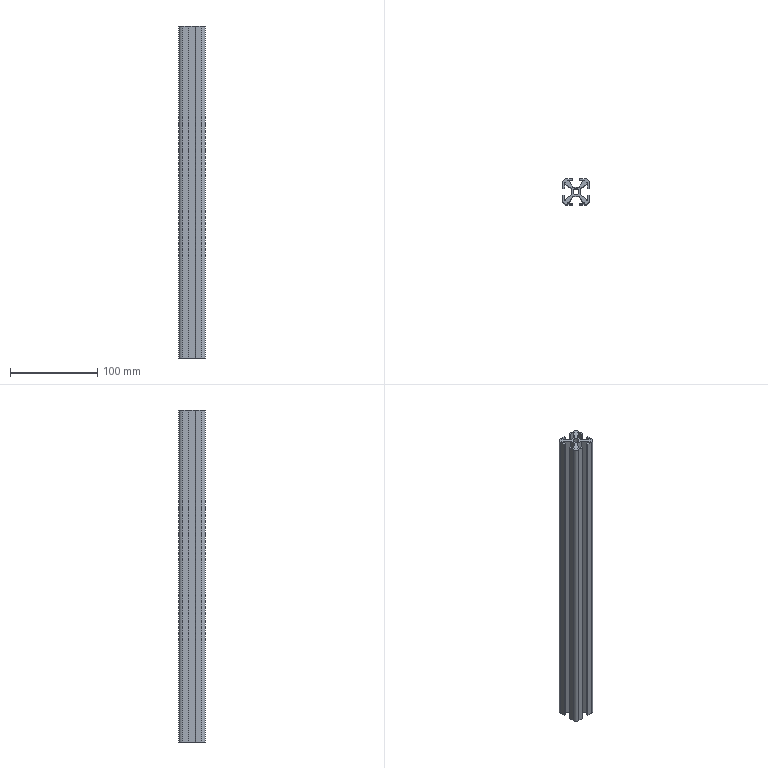Part | SolidWorks | features CirPattern 1, Extrusion 1, Fillet 1, ICE 1 | 1 solid | 60 faces | box 30 x 30 x 380 mm | volume 148880 mm3 | plane 54 | cylinder 6 | commonest cylinder face diameters 9 x4 6.8 x2